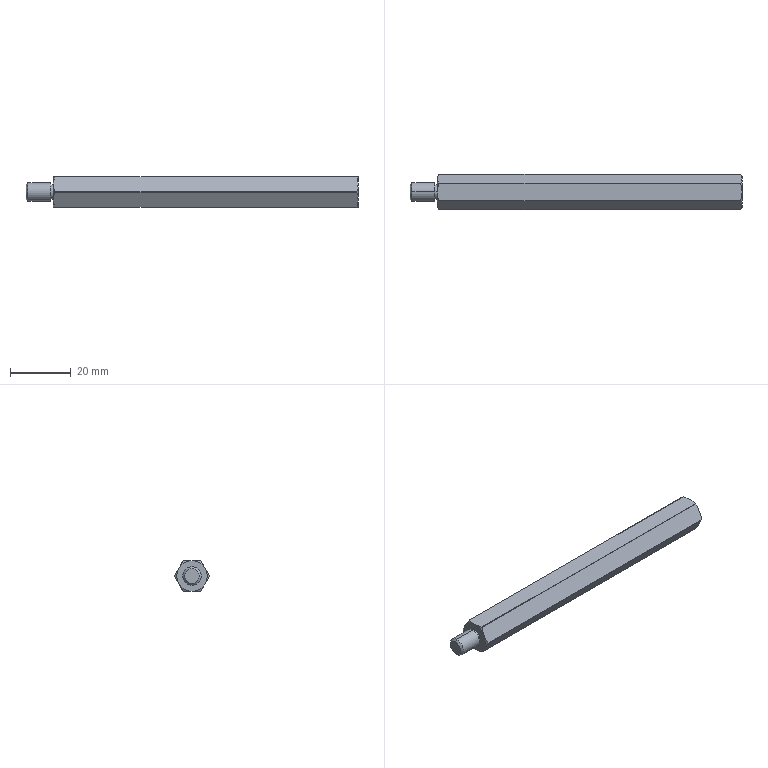Part | STEP file | 0232_014_SLSBWRK10-100 | 1 solid | 40 faces | box 109 x 11.5 x 10 mm | volume 8630 mm3 | cone 18 | cylinder 12 | plane 10 | commonest cylinder face diameters 11.5 x6 4.8 x2 4.917 x2 6 x2